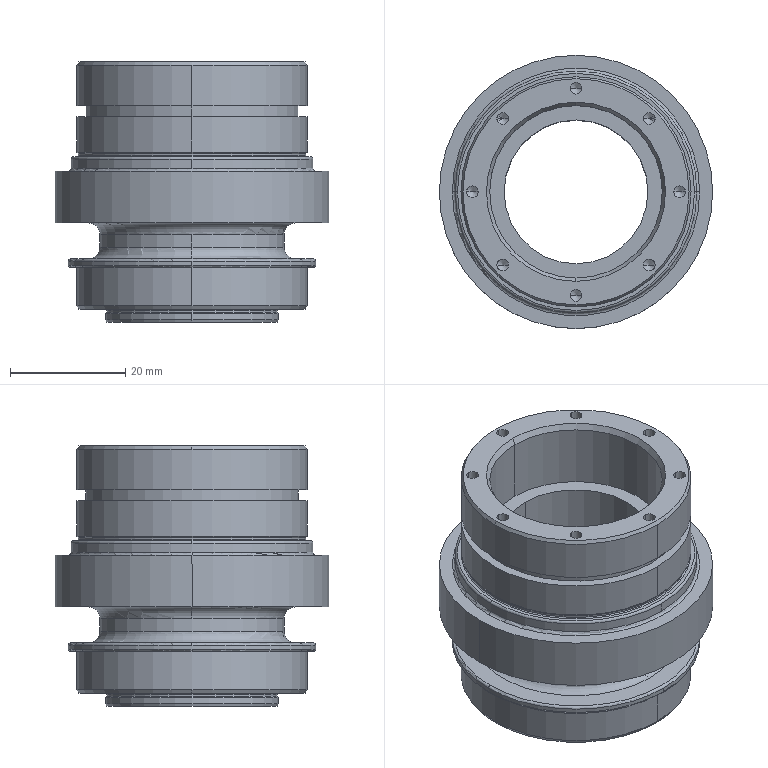Part | SolidWorks | features BaseBody 1 | 1 solid | 131 faces | box 47.505 x 47.505 x 45.25 mm | volume 32627 mm3 | cylinder 58 | cone 46 | torus 16 | plane 11 | commonest cylinder face diameters 2.05 x32 40 x6 30 x4 25 x2 29.6 x2 32 x2